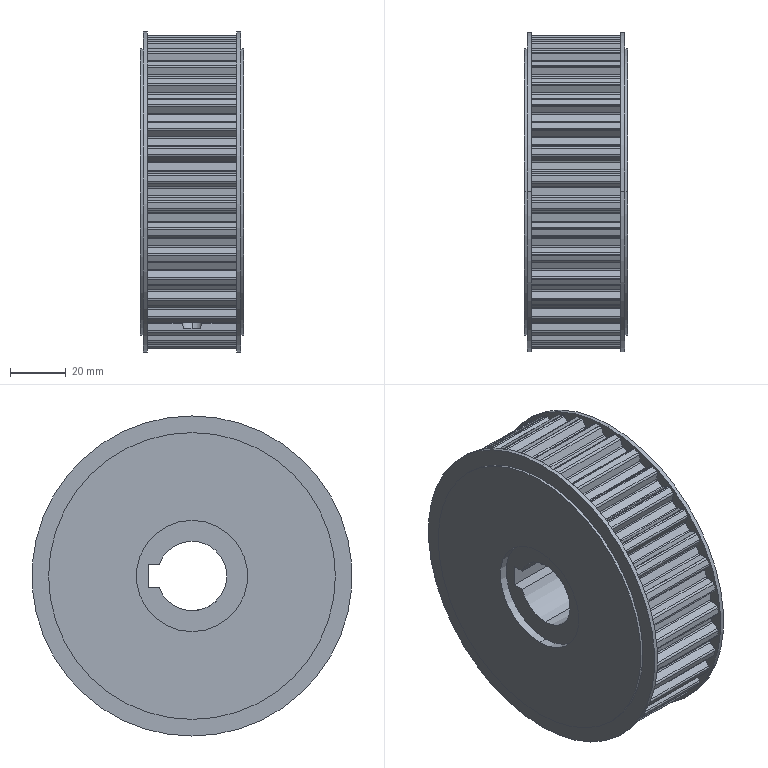Part | SolidWorks | features ICE 8, CirPattern 2, Fillet 2, MirrorPattern 2, Extrusion 1, HoleWzd 1, RevCut 1 | 1 solid | 361 faces | box 37 x 115 x 115 mm | volume 320640 mm3 | cylinder 234 | plane 127 | commonest cylinder face diameters 1.2 x89 1.6 x86 112.74 x36 5 x4 8 x4 40 x4